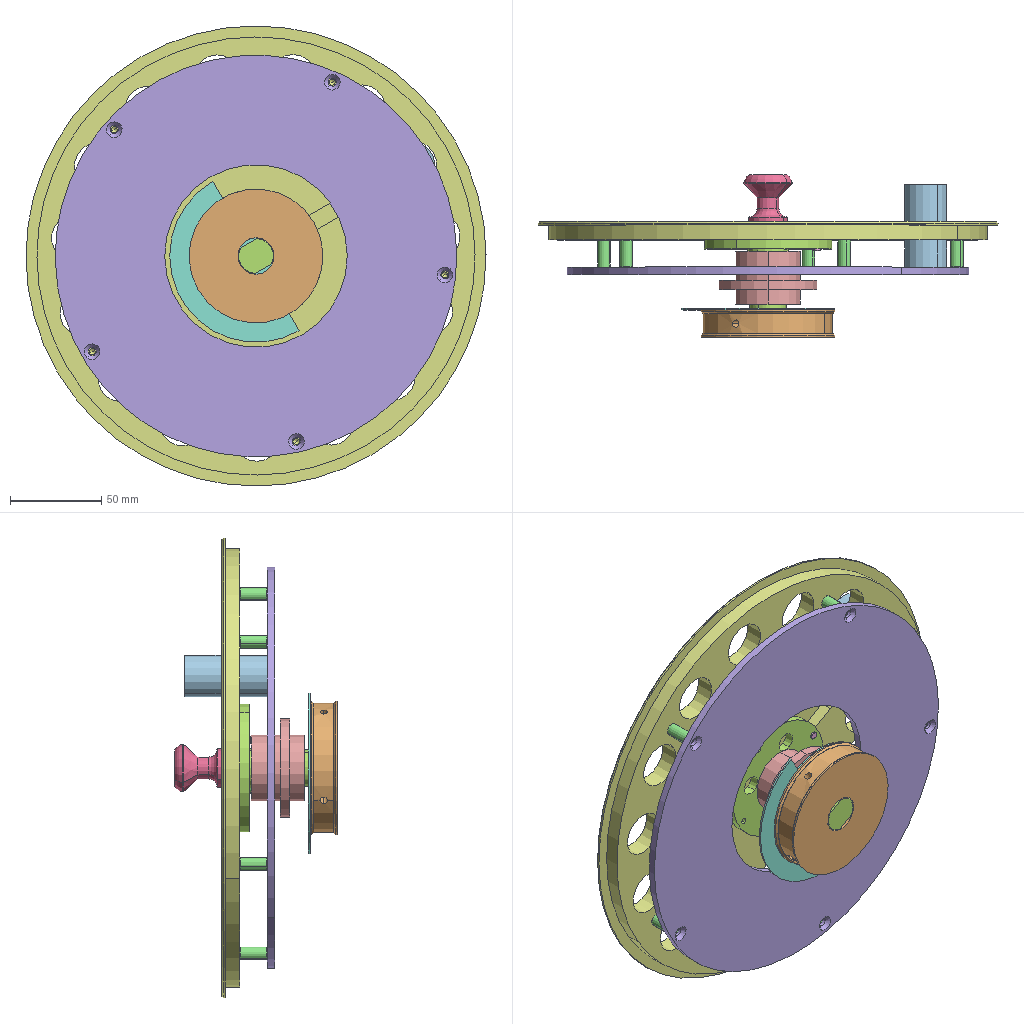Assembly | SolidWorks | 14 different items | 19 placed | box 252 x 89 x 252 mm
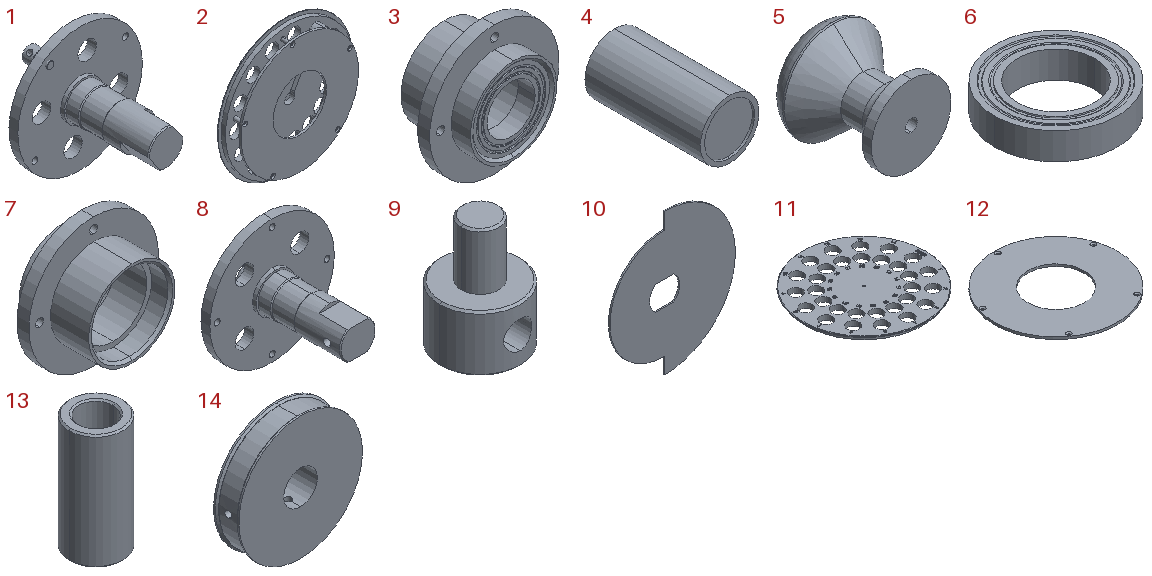Parts list (item | name | quantity | parent item | size | volume | features):
1 | (subassembly) | x1 | - | 70 x 60.9 x 70 mm | 33821 mm3 | -
2 | (subassembly) | x1 | - | 252 x 54.8 x 252 mm | 440411 mm3 | -
3 | (subassembly) | x1 | - | 54 x 29 x 54 mm | 21414 mm3 | -
4 | - | x1 | in 2 | 23 x 45.2 x 23 mm | 3843 mm3 | features ICE 4, Dome 1, Extrusion 1, Shell 1
5 | - | x1 | in 2 | 26.4 x 25.8 x 26.4 mm | 6888 mm3 | features HoleWzd 1, Revolution 1
6 | - | x2 | in 3 | 32 x 32 x 7 mm | 3321 mm3 | features Extrusion 1, MirrorPattern 1, RevCut 1
7 | - | x1 | in 3 | 54 x 29 x 54 mm | 14771 mm3 | features ICE 5, Chamfer 1, Extrusion 1, HoleWzd 1
8 | - | x1 | in 1 | 70 x 60.9 x 70 mm | 33459 mm3 | features ICE 9, Chamfer 2, HoleWzd 2, Extrusion 1
9 | - | x1 | in 1 | 8.6 x 8.6 x 12 mm | 362.769 mm3 | features Chamfer 1, Extrusion 1, HoleWzd 1, ICE 1
10 | - | x1 | - | 83.75 x 1 x 94.5 mm | 5312 mm3 | features ICE 2, Extrusion 1
11 | - | x1 | in 2 | 252 x 252 x 10 mm | 307867 mm3 | features ICE 5, Chamfer 1, Extrusion 1, HoleWzd 1
12 | - | x1 | in 2 | 220 x 220 x 4 mm | 120125 mm3 | features Extrusion 1, HoleWzd 1
13 | - | x5 | in 2 | 7 x 7 x 15 mm | 337.258 mm3 | features Chamfer 1, Extrusion 1
14 | - | x1 | - | 73.4 x 15 x 73.4 mm | 54894 mm3 | features ICE 4, Chamfer 1, Extrusion 1
Mates (type | each side: item.copy, entity, surface, feature):
In the top assembly
Coincident | 8.1 face plane Cut-Extrude3 | 10.1 face plane Boss-Extrude1
Concentric | 8.1 face cylinder Boss-Extrude1 | 10.1 face cylinder Boss-Extrude1
Parallel | 8.1 face plane Cut-Extrude3 | 10.1 face plane Boss-Extrude2
Concentric | 8.1 face cylinder Boss-Extrude1 | 14.1 face cylinder Boss-Extrude1
Parallel | 8.1 face cylinder Cut-Extrude2 | 14.1 face cylinder Cut-Extrude1
Coincident | 8.1 face plane Boss-Extrude1 | 14.1 face plane Boss-Extrude3
Concentric | 8.1 face cylinder Boss-Extrude1 | 6.1 face cylinder Boss-Extrude1
Coincident | 8.1 face plane Boss-Extrude4 | 6.1 face plane Boss-Extrude1
Coincident | 8.1 face plane Boss-Extrude5 | 11.1 face plane Boss-Extrude3
Concentric | 8.1 face cylinder Boss-Extrude6 | 11.1 face cylinder Cut-Extrude4
Tangent | 9.1 face cylinder Boss-Extrude1 | 11.1 face plane Cut-Extrude4
In subassembly 3
Coincident | 7.1 face plane Boss-Extrude2 | 6.2 face plane Boss-Extrude1
Concentric | 7.1 face cylinder Cut-Extrude1 | 6.2 face cylinder Boss-Extrude1
Coincident | 7.1 face plane Cut-Extrude2 | 6.3 face plane Boss-Extrude1
Concentric | 7.1 face cylinder Cut-Extrude2 | 6.3 face cylinder Boss-Extrude1
In subassembly 2
Concentric | 12.1 face cylinder Hole Size (% per cross) Slotted Countersunk Wood Screw Type1 | 13.1 face cylinder Boss-Extrude1
Coincident | 12.1 face plane Boss-Extrude1 | 13.1 face plane Boss-Extrude1
Concentric | 12.1 face cylinder Hole Size (% per cross) Slotted Countersunk Wood Screw Type1 | 13.2 face cylinder Boss-Extrude1
Coincident | 12.1 face plane Boss-Extrude1 | 13.2 face plane Boss-Extrude1
Concentric | 12.1 face cylinder Hole Size (% per cross) Slotted Countersunk Wood Screw Type1 | 13.3 face cylinder Boss-Extrude1
Coincident | 12.1 face plane Boss-Extrude1 | 13.3 face plane Boss-Extrude1
Concentric | 12.1 face cylinder Hole Size (% per cross) Slotted Countersunk Wood Screw Type1 | 13.4 face cylinder Boss-Extrude1
Coincident | 12.1 face plane Boss-Extrude1 | 13.4 face plane Boss-Extrude1
Concentric | 12.1 face cylinder Hole Size (% per cross) Slotted Countersunk Wood Screw Type1 | 13.5 face cylinder Boss-Extrude1
Coincident | 12.1 face plane Boss-Extrude1 | 13.5 face plane Boss-Extrude1
Coincident | 2.1 face | 13.3 face plane Boss-Extrude1
Concentric | 2.1 face | 13.3 face cylinder Boss-Extrude1
Concentric | 2.1 face | 13.5 face cylinder Boss-Extrude1
Coincident | 2.1 face | 5.1 face plane Revolve1
Concentric | 2.1 face | 5.1 face cylinder Revolve1
Coincident | 12.1 face plane Boss-Extrude1 | 4.1 face plane Boss-Extrude1
Concentric | 4.1 face cylinder Boss-Extrude1 | 2.1 face
Coincident | 13.4 face plane Boss-Extrude1 | 11.2 face plane Boss-Extrude3
Concentric | 12.1 face cylinder Boss-Extrude1 | 11.2 face cylinder Boss-Extrude3
Concentric | 13.1 face cylinder Boss-Extrude1 | 11.2 face cylinder M4 Tapped Hole1
Concentric | 4.1 face cylinder Boss-Extrude1 | 11.2 face cylinder Cut-Extrude1
Concentric | 5.1 face cylinder M4 Tapped Hole1 | 11.2 face cylinder Cut-Extrude3
Coincident | 5.1 face plane Revolve1 | 11.2 face plane Boss-Extrude1
In subassembly 1
Coincident | 8.2 face plane Boss-Extrude5 | 9.2 face plane Boss-Extrude1
Concentric | 8.2 face cylinder M4 Tapped Hole3 | 9.2 face cylinder Boss-Extrude1